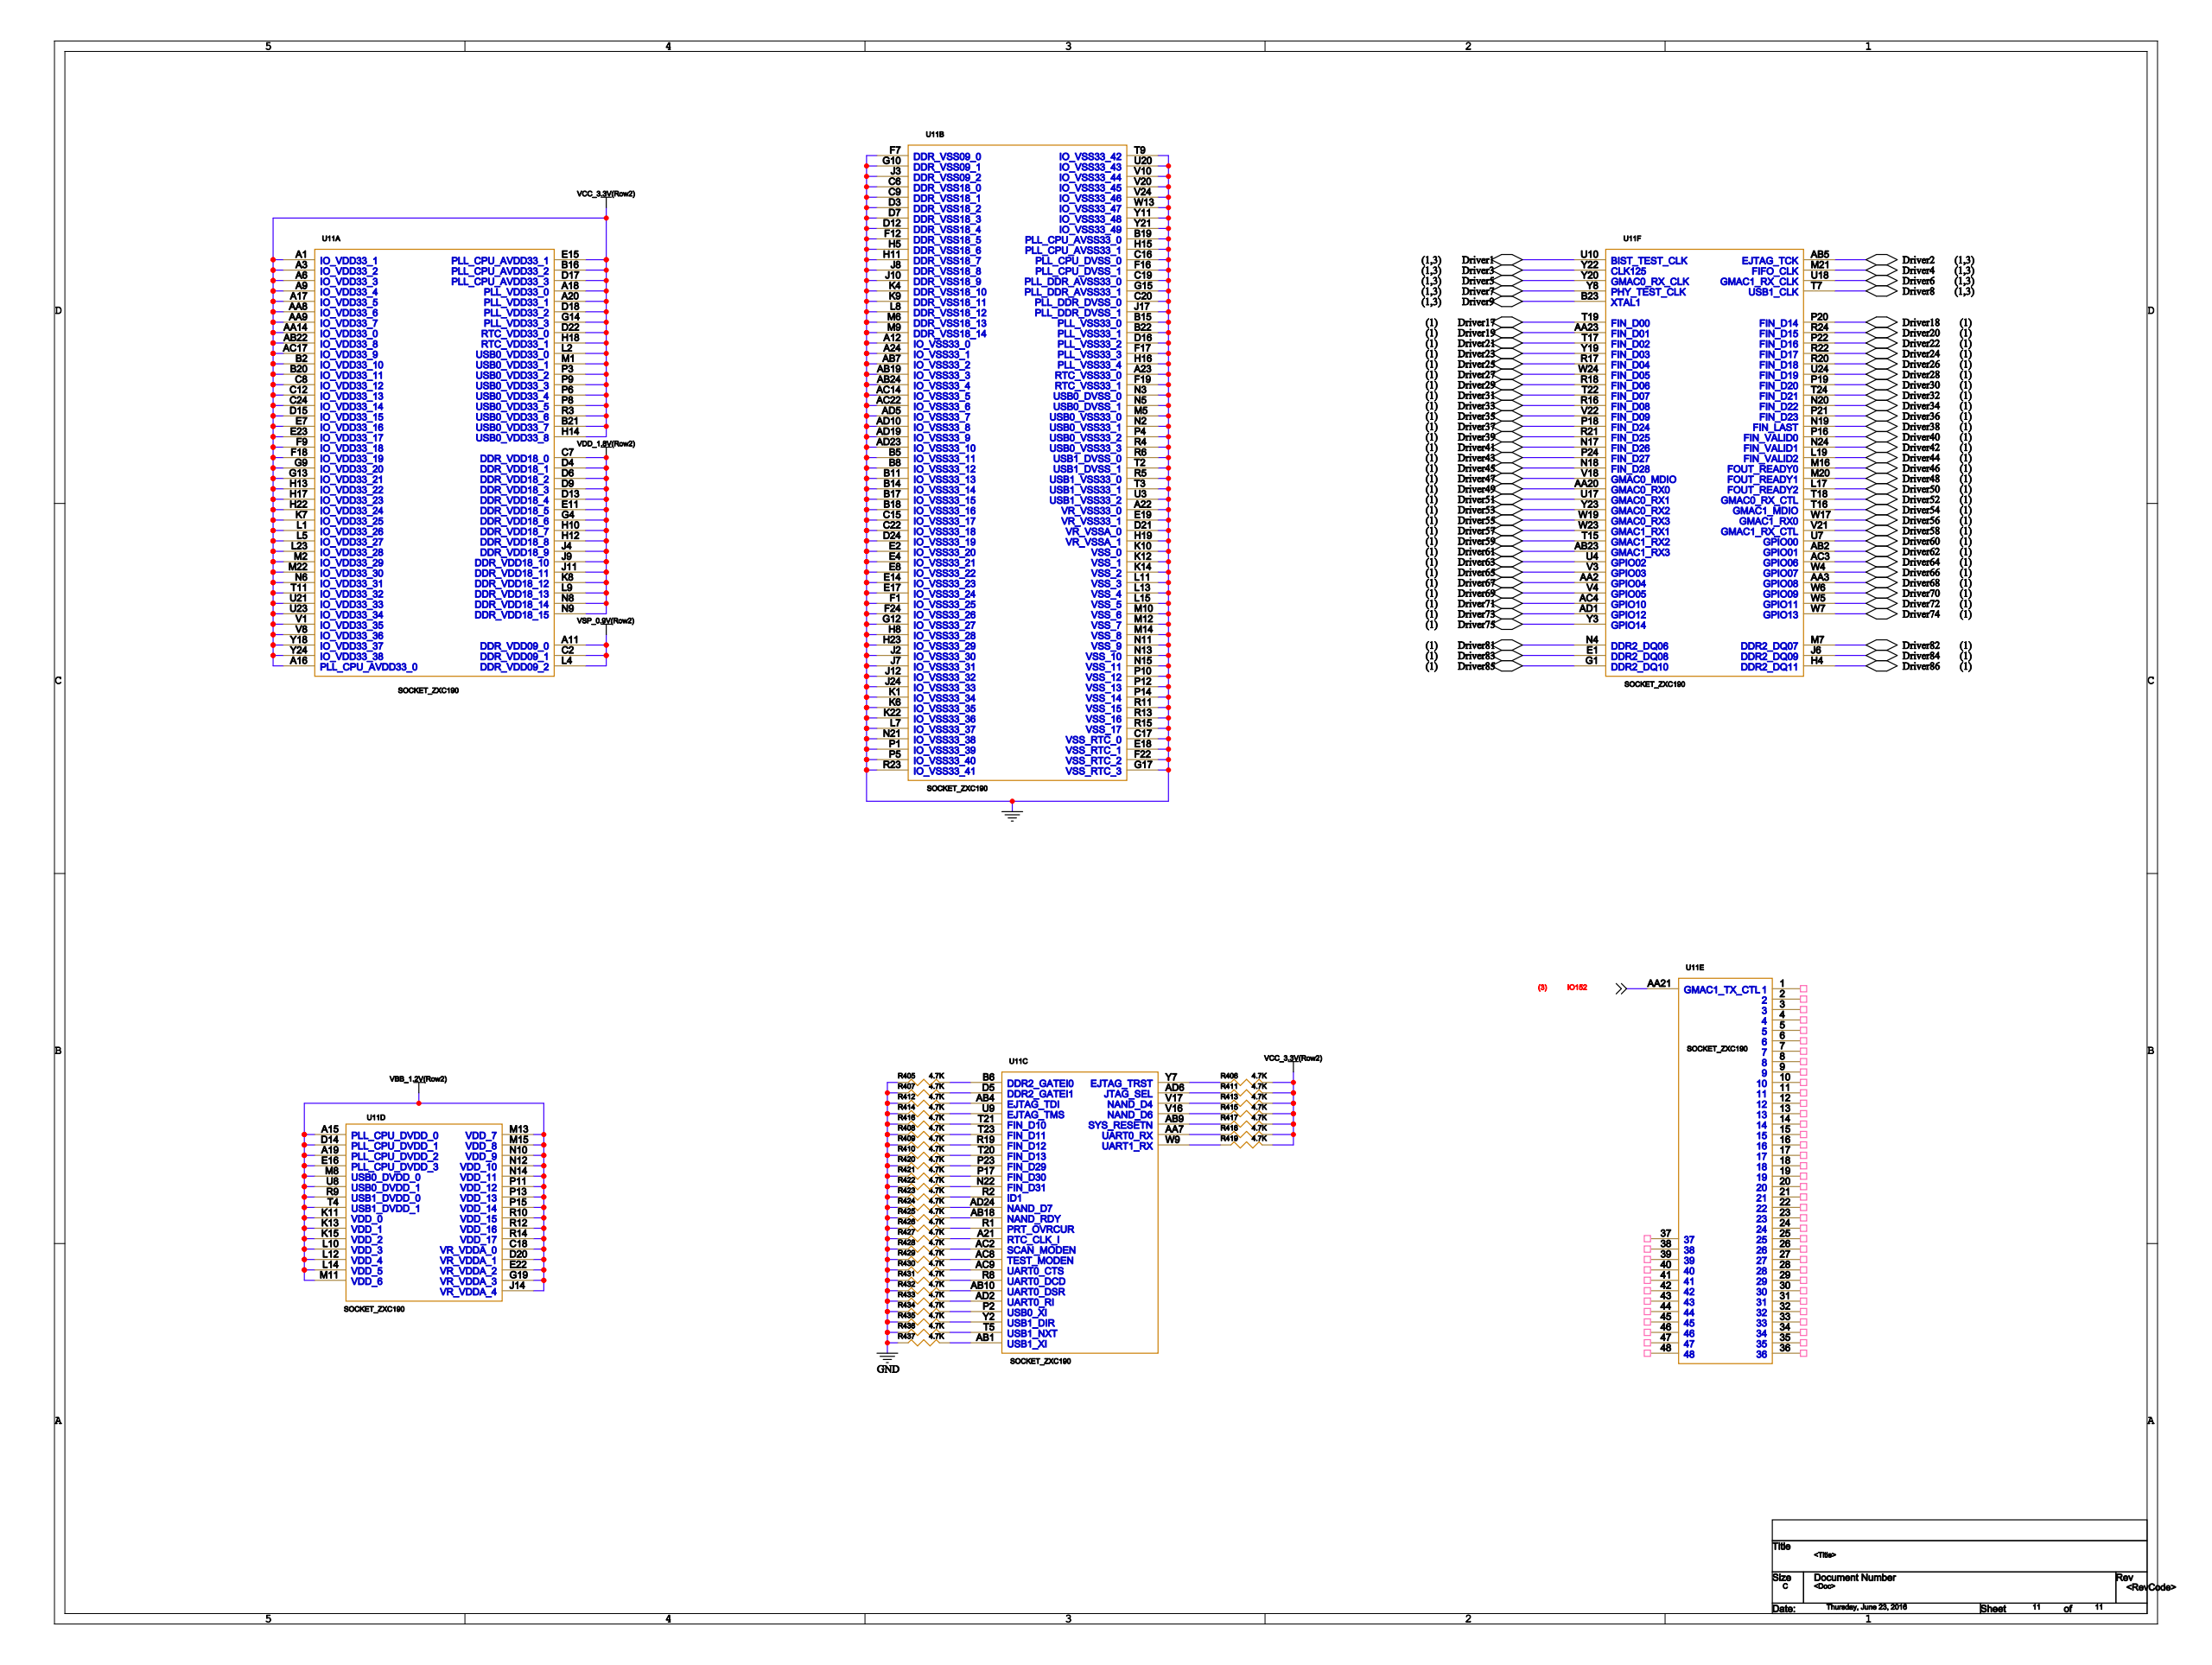Circuit board | Cadence Allegro | 531 parts | 624 nets | one sheet of the schematic
Parts on this sheet (reference | value | footprint):
R405 | 4.7K | R0805
R406 | 4.7K | R0805
R407 | 4.7K | R0805
R408 | 4.7K | R0805
R409 | 4.7K | R0805
R410 | 4.7K | R0805
R411 | 4.7K | R0805
R412 | 4.7K | R0805
R413 | 4.7K | R0805
R414 | 4.7K | R0805
R415 | 4.7K | R0805
R416 | 4.7K | R0805
R417 | 4.7K | R0805
R418 | 4.7K | R0805
R419 | 4.7K | R0805
R420 | 4.7K | R0805
R421 | 4.7K | R0805
R422 | 4.7K | R0805
R423 | 4.7K | R0805
R424 | 4.7K | R0805
R425 | 4.7K | R0805
R426 | 4.7K | R0805
R427 | 4.7K | R0805
R428 | 4.7K | R0805
R429 | 4.7K | R0805
R430 | 4.7K | R0805
R431 | 4.7K | R0805
R432 | 4.7K | R0805
R433 | 4.7K | R0805
R434 | 4.7K | R0805
R435 | 4.7K | R0805
R436 | 4.7K | R0805
R437 | 4.7K | R0805
U3 | SOCKET_ZXC190 | BGA-576
U4 | SOCKET_ZXC190 | BGA-576
U10 | SOCKET_ZXC190 | BGA-576
U11 | SOCKET_ZXC190 | BGA-576
Nets of these parts (net: part-pin ...):
GND: R405-1 R407-1 R408-1 R409-1 R410-1 R412-1 R414-1 R416-1 R420-1 R421-1 R422-1 R423-1 R424-1 R425-1 R426-1 R427-1 R428-1 R429-1 R430-1 R431-1 R432-1 R433-1 R434-1 R435-1 R436-1 R437-1 U3-A12 U3-A22 U3-A23 U3-A24 U3-AB7 U3-AB19 U3-AB24 U3-AC14 U3-AC22 U3-AD5 U3-AD10 U3-AD19 U3-AD23 U3-B5 U3-B8 U3-B11 U3-B14 U3-B15 U3-B17 U3-B18 U3-B19 U3-B22 U3-C6 U3-C9 U3-C15 U3-C16 U3-C17 U3-C19 U3-C20 U3-C22 U3-D3 U3-D7 U3-D12 U3-D16 U3-D21 U3-D24 U3-E2 U3-E4 U3-E8 U3-E14 U3-E17 U3-E18 U3-E19 U3-F1 U3-F7 U3-F12 U3-F16 U3-F17 U3-F19 U3-F22 U3-F24 U3-G10 U3-G12 U3-G15 U3-G17 U3-H5 U3-H8 U3-H11 U3-H15 U3-H16 U3-H19 U3-H23 U3-J2 U3-J3 U3-J7 U3-J8 U3-J10 U3-J12 U3-J17 U3-J24 U3-K1 U3-K4 U3-K6 U3-K9 U3-K10 U3-K12 U3-K14 U3-K22 U3-L7 U3-L8 U3-L11 U3-L13 U3-L15 U3-M5 U3-M6 U3-M9 U3-M10 U3-M12 U3-M14 U3-N2 U3-N3 U3-N5 U3-N11 U3-N13 U3-N15 U3-N21 U3-P1 U3-P4 U3-P5 U3-P10 U3-P12 U3-P14 U3-R4 U3-R5 U3-R6 U3-R11 U3-R13 U3-R15 U3-R23 U3-T2 U3-T3 U3-T9 U3-U3 U3-U20 U3-V10 U3-V20 U3-V24 U3-W13 U3-Y11 U3-Y21 U4-A12 U4-A22 U4-A23 U4-A24 U4-AB7 U4-AB19 U4-AB24 U4-AC14 U4-AC22 U4-AD5 U4-AD10 U4-AD19 U4-AD23 U4-B5 U4-B8 U4-B11 U4-B14 U4-B15 U4-B17 U4-B18 U4-B19 U4-B22 U4-C6 U4-C9 U4-C15 U4-C16 U4-C17 U4-C19 U4-C20 U4-C22 U4-D3 U4-D7 U4-D12 U4-D16 U4-D21 U4-D24 U4-E2 U4-E4 U4-E8 U4-E14 U4-E17 U4-E18 U4-E19 U4-F1 U4-F7 U4-F12 U4-F16 U4-F17 U4-F19 U4-F22 U4-F24 U4-G10 U4-G12 U4-G15 U4-G17 U4-H5 U4-H8 U4-H11 U4-H15 U4-H16 U4-H19 U4-H23 U4-J2 U4-J3 U4-J7 U4-J8 U4-J10 U4-J12 U4-J17 U4-J24 U4-K1 U4-K4 U4-K6 U4-K9 U4-K10 U4-K12 U4-K14 U4-K22 U4-L7 U4-L8 U4-L11 U4-L13 U4-L15 U4-M5 U4-M6 U4-M9 U4-M10 U4-M12 U4-M14 U4-N2 U4-N3 U4-N5 U4-N11 U4-N13 U4-N15 U4-N21 U4-P1 U4-P4 U4-P5 U4-P10 U4-P12 U4-P14 U4-R4 U4-R5 U4-R6 U4-R11 U4-R13 U4-R15 U4-R23 U4-T2 U4-T3 U4-T9 U4-U3 U4-U20 U4-V10 U4-V20 U4-V24 U4-W13 U4-Y11 U4-Y21 U10-A12 U10-A22 U10-A23 U10-A24 U10-AB7 U10-AB19 U10-AB24 U10-AC14 U10-AC22 U10-AD5 U10-AD10 U10-AD19 U10-AD23 U10-B5 U10-B8 U10-B11 U10-B14 U10-B15 U10-B17 U10-B18 U10-B19 U10-B22 U10-C6 U10-C9 U10-C15 U10-C16 U10-C17 U10-C19 U10-C20 U10-C22 U10-D3 U10-D7 U10-D12 U10-D16 U10-D21 U10-D24 U10-E2 U10-E4 U10-E8 U10-E14 U10-E17 U10-E18 U10-E19 U10-F1 U10-F7 U10-F12 U10-F16 U10-F17 U10-F19 U10-F22 U10-F24 U10-G10 U10-G12 U10-G15 U10-G17 U10-H5 U10-H8 U10-H11 U10-H15 U10-H16 U10-H19 U10-H23 U10-J2 U10-J3 U10-J7 U10-J8 U10-J10 U10-J12 U10-J17 U10-J24 U10-K1 U10-K4 U10-K6 U10-K9 U10-K10 U10-K12 U10-K14 U10-K22 U10-L7 U10-L8 U10-L11 U10-L13 U10-L15 U10-M5 U10-M6 U10-M9 U10-M10 U10-M12 U10-M14 U10-N2 U10-N3 U10-N5 U10-N11 U10-N13 U10-N15 U10-N21 U10-P1 U10-P4 U10-P5 U10-P10 U10-P12 U10-P14 U10-R4 U10-R5 U10-R6 U10-R11 U10-R13 U10-R15 U10-R23 U10-T2 U10-T3 U10-T9 U10-U3 U10-U20 U10-V10 U10-V20 U10-V24 U10-W13 U10-Y11 U10-Y21 U11-A12 U11-A22 U11-A23 U11-A24 U11-AB7 U11-AB19 U11-AB24 U11-AC14 U11-AC22 U11-AD5 U11-AD10 U11-AD19 U11-AD23 U11-B5 U11-B8 U11-B11 U11-B14 U11-B15 U11-B17 U11-B18 U11-B19 U11-B22 U11-C6 U11-C9 U11-C15 U11-C16 U11-C17 U11-C19 U11-C20 U11-C22 U11-D3 U11-D7 U11-D12 U11-D16 U11-D21 U11-D24 U11-E2 U11-E4 U11-E8 U11-E14 U11-E17 U11-E18 U11-E19 U11-F1 U11-F7 U11-F12 U11-F16 U11-F17 U11-F19 U11-F22 U11-F24 U11-G10 U11-G12 U11-G15 U11-G17 U11-H5 U11-H8 U11-H11 U11-H15 U11-H16 U11-H19 U11-H23 U11-J2 U11-J3 U11-J7 U11-J8 U11-J10 U11-J12 U11-J17 U11-J24 U11-K1 U11-K4 U11-K6 U11-K9 U11-K10 U11-K12 U11-K14 U11-K22 U11-L7 U11-L8 U11-L11 U11-L13 U11-L15 U11-M5 U11-M6 U11-M9 U11-M10 U11-M12 U11-M14 U11-N2 U11-N3 U11-N5 U11-N11 U11-N13 U11-N15 U11-N21 U11-P1 U11-P4 U11-P5 U11-P10 U11-P12 U11-P14 U11-R4 U11-R5 U11-R6 U11-R11 U11-R13 U11-R15 U11-R23 U11-T2 U11-T3 U11-T9 U11-U3 U11-U20 U11-V10 U11-V20 U11-V24 U11-W13 U11-Y11 U11-Y21
VCC_3.3V(ROW2): R406-2 R411-2 R413-2 R415-2 R417-2 R418-2 R419-2 U10-A1 U10-A3 U10-A6 U10-A9 U10-A16 U10-A17 U10-A18 U10-A20 U10-AA8 U10-AA9 U10-AA14 U10-AB22 U10-AC17 U10-B2 U10-B16 U10-B20 U10-B21 U10-C8 U10-C12 U10-C24 U10-D15 U10-D17 U10-D18 U10-D22 U10-E7 U10-E15 U10-E23 U10-F9 U10-F18 U10-G9 U10-G13 U10-G14 U10-H13 U10-H14 U10-H17 U10-H18 U10-H22 U10-K7 U10-L1 U10-L2 U10-L5 U10-L23 U10-M1 U10-M2 U10-M22 U10-N6 U10-P3 U10-P6 U10-P8 U10-P9 U10-R3 U10-T11 U10-U21 U10-U23 U10-V1 U10-V8 U10-Y18 U10-Y24 U11-A1 U11-A3 U11-A6 U11-A9 U11-A16 U11-A17 U11-A18 U11-A20 U11-AA8 U11-AA9 U11-AA14 U11-AB22 U11-AC17 U11-B2 U11-B16 U11-B20 U11-B21 U11-C8 U11-C12 U11-C24 U11-D15 U11-D17 U11-D18 U11-D22 U11-E7 U11-E15 U11-E23 U11-F9 U11-F18 U11-G9 U11-G13 U11-G14 U11-H13 U11-H14 U11-H17 U11-H18 U11-H22 U11-K7 U11-L1 U11-L2 U11-L5 U11-L23 U11-M1 U11-M2 U11-M22 U11-N6 U11-P3 U11-P6 U11-P8 U11-P9 U11-R3 U11-T11 U11-U21 U11-U23 U11-V1 U11-V8 U11-Y18 U11-Y24
N8586528: R405-2 U11-B6
N8586936: R406-1 U11-Y7
N8586524: R407-2 U11-D5
N8586492: R408-2 U11-T23
N8586488: R409-2 U11-R19
N8586560: R410-2 U11-T20
N8586972: R411-1 U11-AD6
N8586520: R412-2 U11-AB4
N8587132: R413-1 U11-V17
N8586516: R414-2 U11-U9
N8587136: R415-1 U11-V16
N8586512: R416-2 U11-T21
N8587144: R417-1 U11-AB9
N8587140: R418-1 U11-AA7
N8586484: R419-1 U11-W9
N8586556: R420-2 U11-P23
N8586552: R421-2 U11-P17
N8586548: R422-2 U11-N22
N8586544: R423-2 U11-R2
N8586540: R424-2 U11-AD24
N8586536: R425-2 U11-AB18
N8586532: R426-2 U11-R1
N8586588: R427-2 U11-A21
N8586584: R428-2 U11-AC2
N8586580: R429-2 U11-AC8
N8586576: R430-2 U11-AC9
N8587024: R431-2 U11-R8
N8586572: R432-2 U11-AB10
N8586568: R433-2 U11-AD2
N8586564: R434-2 U11-P2
N8586600: R435-2 U11-Y2
N8586596: R436-2 U11-T5
N8586592: R437-2 U11-AB1
IO152: U11-AA21